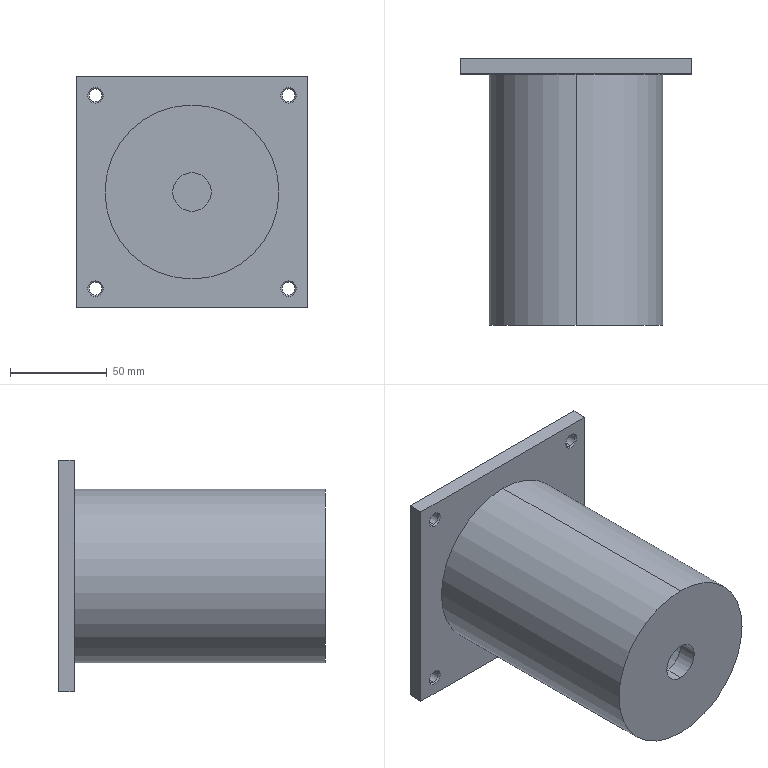Part | SolidWorks | features BaseBody 1 | 1 solid | 39 faces | box 120 x 138 x 120 mm | volume 787135 mm3 | cone 16 | cylinder 14 | plane 9 | commonest cylinder face diameters 6.647 x8 20 x2 40 x2 90 x2
STEP:
#1=CARTESIAN_POINT('',(50.,-0.6765,53.324));
#2=VERTEX_POINT('',#1);
#3=CARTESIAN_POINT('',(50.,-0.6765,46.677));
#4=VERTEX_POINT('',#3);
#5=CARTESIAN_POINT('',(50.,-0.6765,50.));
#6=DIRECTION('',(0.,-1.,0.));
#7=DIRECTION('',(0.,0.,-1.));
#8=AXIS2_PLACEMENT_3D('',#5,#6,#7);
#9=CIRCLE('',#8,3.324);
#10=EDGE_CURVE('',#2,#4,#9,.T.);
#11=ORIENTED_EDGE('',*,*,#10,.T.);
#12=CARTESIAN_POINT('',(50.,0.,46.));
#13=VERTEX_POINT('',#12);
#14=CARTESIAN_POINT('',(50.,0.,46.));
#15=DIRECTION('',(0.,0.7071,-0.7071));
#16=VECTOR('',#15,1000.);
#17=LINE('',#14,#16);
#18=EDGE_CURVE('',#4,#13,#17,.T.);
#19=ORIENTED_EDGE('',*,*,#18,.T.);
#20=CARTESIAN_POINT('',(50.,0.,54.));
#21=VERTEX_POINT('',#20);
#22=CARTESIAN_POINT('',(50.,0.,50.));
#23=DIRECTION('',(0.,-1.,0.));
#24=DIRECTION('',(0.,0.,-1.));
#25=AXIS2_PLACEMENT_3D('',#22,#23,#24);
#26=CIRCLE('',#25,4.);
#27=EDGE_CURVE('',#21,#13,#26,.T.);
#28=ORIENTED_EDGE('',*,*,#27,.F.);
#29=CARTESIAN_POINT('',(50.,0.,54.));
#30=DIRECTION('',(0.,0.7071,0.7071));
#31=VECTOR('',#30,1000.);
#32=LINE('',#29,#31);
#33=EDGE_CURVE('',#2,#21,#32,.T.);
#34=ORIENTED_EDGE('',*,*,#33,.F.);
#35=EDGE_LOOP('',(#11,#19,#28,#34));
#36=FACE_OUTER_BOUND('',#35,.T.);
#37=CARTESIAN_POINT('',(50.,0.,50.));
#38=DIRECTION('',(0.,1.,0.));
#39=DIRECTION('',(0.,0.,1.));
#40=AXIS2_PLACEMENT_3D('',#37,#38,#39);
#41=CONICAL_SURFACE('',#40,4.,0.7854);
#42=ADVANCED_FACE('',(#36),#41,.F.);
#43=CARTESIAN_POINT('',(-50.,-0.6765,53.324));
#44=VERTEX_POINT('',#43);
#45=CARTESIAN_POINT('',(-50.,-0.6765,46.677));
#46=VERTEX_POINT('',#45);
#47=CARTESIAN_POINT('',(-50.,-0.6765,50.));
#48=DIRECTION('',(0.,-1.,0.));
#49=DIRECTION('',(0.,0.,-1.));
#50=AXIS2_PLACEMENT_3D('',#47,#48,#49);
#51=CIRCLE('',#50,3.324);
#52=EDGE_CURVE('',#44,#46,#51,.T.);
#53=ORIENTED_EDGE('',*,*,#52,.T.);
#54=CARTESIAN_POINT('',(-50.,0.,46.));
#55=VERTEX_POINT('',#54);
#56=CARTESIAN_POINT('',(-50.,0.,46.));
#57=DIRECTION('',(0.,0.7071,-0.7071));
#58=VECTOR('',#57,1000.);
#59=LINE('',#56,#58);
#60=EDGE_CURVE('',#46,#55,#59,.T.);
#61=ORIENTED_EDGE('',*,*,#60,.T.);
#62=CARTESIAN_POINT('',(-50.,0.,54.));
#63=VERTEX_POINT('',#62);
#64=CARTESIAN_POINT('',(-50.,0.,50.));
#65=DIRECTION('',(0.,-1.,0.));
#66=DIRECTION('',(0.,0.,-1.));
#67=AXIS2_PLACEMENT_3D('',#64,#65,#66);
#68=CIRCLE('',#67,4.);
#69=EDGE_CURVE('',#63,#55,#68,.T.);
#70=ORIENTED_EDGE('',*,*,#69,.F.);
#71=CARTESIAN_POINT('',(-50.,0.,54.));
#72=DIRECTION('',(0.,0.7071,0.7071));
#73=VECTOR('',#72,1000.);
#74=LINE('',#71,#73);
#75=EDGE_CURVE('',#44,#63,#74,.T.);
#76=ORIENTED_EDGE('',*,*,#75,.F.);
#77=EDGE_LOOP('',(#53,#61,#70,#76));
#78=FACE_OUTER_BOUND('',#77,.T.);
#79=CARTESIAN_POINT('',(-50.,0.,50.));
#80=DIRECTION('',(0.,1.,0.));
#81=DIRECTION('',(0.,0.,1.));
#82=AXIS2_PLACEMENT_3D('',#79,#80,#81);
#83=CONICAL_SURFACE('',#82,4.,0.7854);
#84=ADVANCED_FACE('',(#78),#83,.F.);
#85=CARTESIAN_POINT('',(-50.,-0.6765,-46.677));
#86=VERTEX_POINT('',#85);
#87=CARTESIAN_POINT('',(-50.,-0.6765,-53.324));
#88=VERTEX_POINT('',#87);
#89=CARTESIAN_POINT('',(-50.,-0.6765,-50.));
#90=DIRECTION('',(0.,-1.,0.));
#91=DIRECTION('',(0.,0.,-1.));
#92=AXIS2_PLACEMENT_3D('',#89,#90,#91);
#93=CIRCLE('',#92,3.324);
#94=EDGE_CURVE('',#86,#88,#93,.T.);
#95=ORIENTED_EDGE('',*,*,#94,.T.);
#96=CARTESIAN_POINT('',(-50.,0.,-54.));
#97=VERTEX_POINT('',#96);
#98=CARTESIAN_POINT('',(-50.,0.,-54.));
#99=DIRECTION('',(0.,0.7071,-0.7071));
#100=VECTOR('',#99,1000.);
#101=LINE('',#98,#100);
#102=EDGE_CURVE('',#88,#97,#101,.T.);
#103=ORIENTED_EDGE('',*,*,#102,.T.);
#104=CARTESIAN_POINT('',(-50.,0.,-46.));
#105=VERTEX_POINT('',#104);
#106=CARTESIAN_POINT('',(-50.,0.,-50.));
#107=DIRECTION('',(0.,-1.,0.));
#108=DIRECTION('',(0.,0.,-1.));
#109=AXIS2_PLACEMENT_3D('',#106,#107,#108);
#110=CIRCLE('',#109,4.);
#111=EDGE_CURVE('',#105,#97,#110,.T.);
#112=ORIENTED_EDGE('',*,*,#111,.F.);
#113=CARTESIAN_POINT('',(-50.,0.,-46.));
#114=DIRECTION('',(0.,0.7071,0.7071));
#115=VECTOR('',#114,1000.);
#116=LINE('',#113,#115);
#117=EDGE_CURVE('',#86,#105,#116,.T.);
#118=ORIENTED_EDGE('',*,*,#117,.F.);
#119=EDGE_LOOP('',(#95,#103,#112,#118));
#120=FACE_OUTER_BOUND('',#119,.T.);
#121=CARTESIAN_POINT('',(-50.,0.,-50.));
#122=DIRECTION('',(0.,1.,0.));
#123=DIRECTION('',(0.,0.,1.));
#124=AXIS2_PLACEMENT_3D('',#121,#122,#123);
#125=CONICAL_SURFACE('',#124,4.,0.7854);
#126=ADVANCED_FACE('',(#120),#125,.F.);
#127=CARTESIAN_POINT('',(50.,-0.6765,-46.677));
#128=VERTEX_POINT('',#127);
#129=CARTESIAN_POINT('',(50.,-0.6765,-53.324));
#130=VERTEX_POINT('',#129);
#131=CARTESIAN_POINT('',(50.,-0.6765,-50.));
#132=DIRECTION('',(0.,-1.,0.));
#133=DIRECTION('',(0.,0.,-1.));
#134=AXIS2_PLACEMENT_3D('',#131,#132,#133);
#135=CIRCLE('',#134,3.324);
#136=EDGE_CURVE('',#128,#130,#135,.T.);
#137=ORIENTED_EDGE('',*,*,#136,.T.);
#138=CARTESIAN_POINT('',(50.,0.,-54.));
#139=VERTEX_POINT('',#138);
#140=CARTESIAN_POINT('',(50.,0.,-54.));
#141=DIRECTION('',(0.,0.7071,-0.7071));
#142=VECTOR('',#141,1000.);
#143=LINE('',#140,#142);
#144=EDGE_CURVE('',#130,#139,#143,.T.);
#145=ORIENTED_EDGE('',*,*,#144,.T.);
#146=CARTESIAN_POINT('',(50.,0.,-46.));
#147=VERTEX_POINT('',#146);
#148=CARTESIAN_POINT('',(50.,0.,-50.));
#149=DIRECTION('',(0.,-1.,0.));
#150=DIRECTION('',(0.,0.,-1.));
#151=AXIS2_PLACEMENT_3D('',#148,#149,#150);
#152=CIRCLE('',#151,4.);
#153=EDGE_CURVE('',#147,#139,#152,.T.);
#154=ORIENTED_EDGE('',*,*,#153,.F.);
#155=CARTESIAN_POINT('',(50.,0.,-46.));
#156=DIRECTION('',(0.,0.7071,0.7071));
#157=VECTOR('',#156,1000.);
#158=LINE('',#155,#157);
#159=EDGE_CURVE('',#128,#147,#158,.T.);
#160=ORIENTED_EDGE('',*,*,#159,.F.);
#161=EDGE_LOOP('',(#137,#145,#154,#160));
#162=FACE_OUTER_BOUND('',#161,.T.);
#163=CARTESIAN_POINT('',(50.,0.,-50.));
#164=DIRECTION('',(0.,1.,0.));
#165=DIRECTION('',(0.,0.,1.));
#166=AXIS2_PLACEMENT_3D('',#163,#164,#165);
#167=CONICAL_SURFACE('',#166,4.,0.7854);
#168=ADVANCED_FACE('',(#162),#167,.F.);
#169=ORIENTED_EDGE('',*,*,#10,.F.);
#170=CARTESIAN_POINT('',(50.,-7.324,53.324));
#171=VERTEX_POINT('',#170);
#172=CARTESIAN_POINT('',(50.,-8.,53.324));
#173=DIRECTION('',(0.,-1.,0.));
#174=VECTOR('',#173,1000.);
#175=LINE('',#172,#174);
#176=EDGE_CURVE('',#2,#171,#175,.T.);
#177=ORIENTED_EDGE('',*,*,#176,.T.);
#178=CARTESIAN_POINT('',(50.,-7.324,46.677));
#179=VERTEX_POINT('',#178);
#180=CARTESIAN_POINT('',(50.,-7.324,50.));
#181=DIRECTION('',(0.,-1.,0.));
#182=DIRECTION('',(0.,0.,-1.));
#183=AXIS2_PLACEMENT_3D('',#180,#181,#182);
#184=CIRCLE('',#183,3.324);
#185=EDGE_CURVE('',#171,#179,#184,.T.);
#186=ORIENTED_EDGE('',*,*,#185,.T.);
#187=CARTESIAN_POINT('',(50.,-8.,46.677));
#188=DIRECTION('',(0.,-1.,0.));
#189=VECTOR('',#188,1000.);
#190=LINE('',#187,#189);
#191=EDGE_CURVE('',#4,#179,#190,.T.);
#192=ORIENTED_EDGE('',*,*,#191,.F.);
#193=EDGE_LOOP('',(#169,#177,#186,#192));
#194=FACE_OUTER_BOUND('',#193,.T.);
#195=CARTESIAN_POINT('',(50.,-8.,50.));
#196=DIRECTION('',(0.,-1.,0.));
#197=DIRECTION('',(0.,0.,-1.));
#198=AXIS2_PLACEMENT_3D('',#195,#196,#197);
#199=CYLINDRICAL_SURFACE('',#198,3.324);
#200=ADVANCED_FACE('',(#194),#199,.F.);
#201=ORIENTED_EDGE('',*,*,#52,.F.);
#202=CARTESIAN_POINT('',(-50.,-7.324,53.324));
#203=VERTEX_POINT('',#202);
#204=CARTESIAN_POINT('',(-50.,-8.,53.324));
#205=DIRECTION('',(0.,-1.,0.));
#206=VECTOR('',#205,1000.);
#207=LINE('',#204,#206);
#208=EDGE_CURVE('',#44,#203,#207,.T.);
#209=ORIENTED_EDGE('',*,*,#208,.T.);
#210=CARTESIAN_POINT('',(-50.,-7.324,46.677));
#211=VERTEX_POINT('',#210);
#212=CARTESIAN_POINT('',(-50.,-7.324,50.));
#213=DIRECTION('',(0.,-1.,0.));
#214=DIRECTION('',(0.,0.,-1.));
#215=AXIS2_PLACEMENT_3D('',#212,#213,#214);
#216=CIRCLE('',#215,3.324);
#217=EDGE_CURVE('',#203,#211,#216,.T.);
#218=ORIENTED_EDGE('',*,*,#217,.T.);
#219=CARTESIAN_POINT('',(-50.,-8.,46.677));
#220=DIRECTION('',(0.,-1.,0.));
#221=VECTOR('',#220,1000.);
#222=LINE('',#219,#221);
#223=EDGE_CURVE('',#46,#211,#222,.T.);
#224=ORIENTED_EDGE('',*,*,#223,.F.);
#225=EDGE_LOOP('',(#201,#209,#218,#224));
#226=FACE_OUTER_BOUND('',#225,.T.);
#227=CARTESIAN_POINT('',(-50.,-8.,50.));
#228=DIRECTION('',(0.,-1.,0.));
#229=DIRECTION('',(0.,0.,-1.));
#230=AXIS2_PLACEMENT_3D('',#227,#228,#229);
#231=CYLINDRICAL_SURFACE('',#230,3.324);
#232=ADVANCED_FACE('',(#226),#231,.F.);
#233=ORIENTED_EDGE('',*,*,#94,.F.);
#234=CARTESIAN_POINT('',(-50.,-7.324,-46.677));
#235=VERTEX_POINT('',#234);
#236=CARTESIAN_POINT('',(-50.,-8.,-46.677));
#237=DIRECTION('',(0.,-1.,0.));
#238=VECTOR('',#237,1000.);
#239=LINE('',#236,#238);
#240=EDGE_CURVE('',#86,#235,#239,.T.);
#241=ORIENTED_EDGE('',*,*,#240,.T.);
#242=CARTESIAN_POINT('',(-50.,-7.324,-53.324));
#243=VERTEX_POINT('',#242);
#244=CARTESIAN_POINT('',(-50.,-7.324,-50.));
#245=DIRECTION('',(0.,-1.,0.));
#246=DIRECTION('',(0.,0.,-1.));
#247=AXIS2_PLACEMENT_3D('',#244,#245,#246);
#248=CIRCLE('',#247,3.324);
#249=EDGE_CURVE('',#235,#243,#248,.T.);
#250=ORIENTED_EDGE('',*,*,#249,.T.);
#251=CARTESIAN_POINT('',(-50.,-8.,-53.324));
#252=DIRECTION('',(0.,-1.,0.));
#253=VECTOR('',#252,1000.);
#254=LINE('',#251,#253);
#255=EDGE_CURVE('',#88,#243,#254,.T.);
#256=ORIENTED_EDGE('',*,*,#255,.F.);
#257=EDGE_LOOP('',(#233,#241,#250,#256));
#258=FACE_OUTER_BOUND('',#257,.T.);
#259=CARTESIAN_POINT('',(-50.,-8.,-50.));
#260=DIRECTION('',(0.,-1.,0.));
#261=DIRECTION('',(0.,0.,-1.));
#262=AXIS2_PLACEMENT_3D('',#259,#260,#261);
#263=CYLINDRICAL_SURFACE('',#262,3.324);
#264=ADVANCED_FACE('',(#258),#263,.F.);
#265=ORIENTED_EDGE('',*,*,#136,.F.);
#266=CARTESIAN_POINT('',(50.,-7.324,-46.677));
#267=VERTEX_POINT('',#266);
#268=CARTESIAN_POINT('',(50.,-8.,-46.677));
#269=DIRECTION('',(0.,-1.,0.));
#270=VECTOR('',#269,1000.);
#271=LINE('',#268,#270);
#272=EDGE_CURVE('',#128,#267,#271,.T.);
#273=ORIENTED_EDGE('',*,*,#272,.T.);
#274=CARTESIAN_POINT('',(50.,-7.324,-53.324));
#275=VERTEX_POINT('',#274);
#276=CARTESIAN_POINT('',(50.,-7.324,-50.));
#277=DIRECTION('',(0.,-1.,0.));
#278=DIRECTION('',(0.,0.,-1.));
#279=AXIS2_PLACEMENT_3D('',#276,#277,#278);
#280=CIRCLE('',#279,3.324);
#281=EDGE_CURVE('',#267,#275,#280,.T.);
#282=ORIENTED_EDGE('',*,*,#281,.T.);
#283=CARTESIAN_POINT('',(50.,-8.,-53.324));
#284=DIRECTION('',(0.,-1.,0.));
#285=VECTOR('',#284,1000.);
#286=LINE('',#283,#285);
#287=EDGE_CURVE('',#130,#275,#286,.T.);
#288=ORIENTED_EDGE('',*,*,#287,.F.);
#289=EDGE_LOOP('',(#265,#273,#282,#288));
#290=FACE_OUTER_BOUND('',#289,.T.);
#291=CARTESIAN_POINT('',(50.,-8.,-50.));
#292=DIRECTION('',(0.,-1.,0.));
#293=DIRECTION('',(0.,0.,-1.));
#294=AXIS2_PLACEMENT_3D('',#291,#292,#293);
#295=CYLINDRICAL_SURFACE('',#294,3.324);
#296=ADVANCED_FACE('',(#290),#295,.F.);
#297=ORIENTED_EDGE('',*,*,#185,.F.);
#298=CARTESIAN_POINT('',(50.,-8.,54.));
#299=VERTEX_POINT('',#298);
#300=CARTESIAN_POINT('',(50.,-7.324,53.324));
#301=DIRECTION('',(0.,-0.7071,0.7071));
#302=VECTOR('',#301,1000.);
#303=LINE('',#300,#302);
#304=EDGE_CURVE('',#171,#299,#303,.T.);
#305=ORIENTED_EDGE('',*,*,#304,.T.);
#306=CARTESIAN_POINT('',(50.,-8.,46.));
#307=VERTEX_POINT('',#306);
#308=CARTESIAN_POINT('',(50.,-8.,50.));
#309=DIRECTION('',(0.,-1.,0.));
#310=DIRECTION('',(0.,0.,-1.));
#311=AXIS2_PLACEMENT_3D('',#308,#309,#310);
#312=CIRCLE('',#311,4.);
#313=EDGE_CURVE('',#299,#307,#312,.T.);
#314=ORIENTED_EDGE('',*,*,#313,.T.);
#315=CARTESIAN_POINT('',(50.,-7.324,46.677));
#316=DIRECTION('',(0.,-0.7071,-0.7071));
#317=VECTOR('',#316,1000.);
#318=LINE('',#315,#317);
#319=EDGE_CURVE('',#179,#307,#318,.T.);
#320=ORIENTED_EDGE('',*,*,#319,.F.);
#321=EDGE_LOOP('',(#297,#305,#314,#320));
#322=FACE_OUTER_BOUND('',#321,.T.);
#323=CARTESIAN_POINT('',(50.,-7.324,50.));
#324=DIRECTION('',(0.,-1.,0.));
#325=DIRECTION('',(0.,0.,-1.));
#326=AXIS2_PLACEMENT_3D('',#323,#324,#325);
#327=CONICAL_SURFACE('',#326,3.324,0.7854);
#328=ADVANCED_FACE('',(#322),#327,.F.);
#329=ORIENTED_EDGE('',*,*,#217,.F.);
#330=CARTESIAN_POINT('',(-50.,-8.,54.));
#331=VERTEX_POINT('',#330);
#332=CARTESIAN_POINT('',(-50.,-7.324,53.324));
#333=DIRECTION('',(0.,-0.7071,0.7071));
#334=VECTOR('',#333,1000.);
#335=LINE('',#332,#334);
#336=EDGE_CURVE('',#203,#331,#335,.T.);
#337=ORIENTED_EDGE('',*,*,#336,.T.);
#338=CARTESIAN_POINT('',(-50.,-8.,46.));
#339=VERTEX_POINT('',#338);
#340=CARTESIAN_POINT('',(-50.,-8.,50.));
#341=DIRECTION('',(0.,-1.,0.));
#342=DIRECTION('',(0.,0.,-1.));
#343=AXIS2_PLACEMENT_3D('',#340,#341,#342);
#344=CIRCLE('',#343,4.);
#345=EDGE_CURVE('',#331,#339,#344,.T.);
#346=ORIENTED_EDGE('',*,*,#345,.T.);
#347=CARTESIAN_POINT('',(-50.,-7.324,46.677));
#348=DIRECTION('',(0.,-0.7071,-0.7071));
#349=VECTOR('',#348,1000.);
#350=LINE('',#347,#349);
#351=EDGE_CURVE('',#211,#339,#350,.T.);
#352=ORIENTED_EDGE('',*,*,#351,.F.);
#353=EDGE_LOOP('',(#329,#337,#346,#352));
#354=FACE_OUTER_BOUND('',#353,.T.);
#355=CARTESIAN_POINT('',(-50.,-7.324,50.));
#356=DIRECTION('',(0.,-1.,0.));
#357=DIRECTION('',(0.,0.,-1.));
#358=AXIS2_PLACEMENT_3D('',#355,#356,#357);
#359=CONICAL_SURFACE('',#358,3.324,0.7854);
#360=ADVANCED_FACE('',(#354),#359,.F.);
#361=ORIENTED_EDGE('',*,*,#249,.F.);
#362=CARTESIAN_POINT('',(-50.,-8.,-46.));
#363=VERTEX_POINT('',#362);
#364=CARTESIAN_POINT('',(-50.,-7.324,-46.677));
#365=DIRECTION('',(0.,-0.7071,0.7071));
#366=VECTOR('',#365,1000.);
#367=LINE('',#364,#366);
#368=EDGE_CURVE('',#235,#363,#367,.T.);
#369=ORIENTED_EDGE('',*,*,#368,.T.);
#370=CARTESIAN_POINT('',(-50.,-8.,-54.));
#371=VERTEX_POINT('',#370);
#372=CARTESIAN_POINT('',(-50.,-8.,-50.));
#373=DIRECTION('',(0.,-1.,0.));
#374=DIRECTION('',(0.,0.,-1.));
#375=AXIS2_PLACEMENT_3D('',#372,#373,#374);
#376=CIRCLE('',#375,4.);
#377=EDGE_CURVE('',#363,#371,#376,.T.);
#378=ORIENTED_EDGE('',*,*,#377,.T.);
#379=CARTESIAN_POINT('',(-50.,-7.324,-53.324));
#380=DIRECTION('',(0.,-0.7071,-0.7071));
#381=VECTOR('',#380,1000.);
#382=LINE('',#379,#381);
#383=EDGE_CURVE('',#243,#371,#382,.T.);
#384=ORIENTED_EDGE('',*,*,#383,.F.);
#385=EDGE_LOOP('',(#361,#369,#378,#384));
#386=FACE_OUTER_BOUND('',#385,.T.);
#387=CARTESIAN_POINT('',(-50.,-7.324,-50.));
#388=DIRECTION('',(0.,-1.,0.));
#389=DIRECTION('',(0.,0.,-1.));
#390=AXIS2_PLACEMENT_3D('',#387,#388,#389);
#391=CONICAL_SURFACE('',#390,3.324,0.7854);
#392=ADVANCED_FACE('',(#386),#391,.F.);
#393=ORIENTED_EDGE('',*,*,#281,.F.);
#394=CARTESIAN_POINT('',(50.,-8.,-46.));
#395=VERTEX_POINT('',#394);
#396=CARTESIAN_POINT('',(50.,-7.324,-46.677));
#397=DIRECTION('',(0.,-0.7071,0.7071));
#398=VECTOR('',#397,1000.);
#399=LINE('',#396,#398);
#400=EDGE_CURVE('',#267,#395,#399,.T.);
#401=ORIENTED_EDGE('',*,*,#400,.T.);
#402=CARTESIAN_POINT('',(50.,-8.,-54.));
#403=VERTEX_POINT('',#402);
#404=CARTESIAN_POINT('',(50.,-8.,-50.));
#405=DIRECTION('',(0.,-1.,0.));
#406=DIRECTION('',(0.,0.,-1.));
#407=AXIS2_PLACEMENT_3D('',#404,#405,#406);
#408=CIRCLE('',#407,4.);
#409=EDGE_CURVE('',#395,#403,#408,.T.);
#410=ORIENTED_EDGE('',*,*,#409,.T.);
#411=CARTESIAN_POINT('',(50.,-7.324,-53.324));
#412=DIRECTION('',(0.,-0.7071,-0.7071));
#413=VECTOR('',#412,1000.);
#414=LINE('',#411,#413);
#415=EDGE_CURVE('',#275,#403,#414,.T.);
#416=ORIENTED_EDGE('',*,*,#415,.F.);
#417=EDGE_LOOP('',(#393,#401,#410,#416));
#418=FACE_OUTER_BOUND('',#417,.T.);
#419=CARTESIAN_POINT('',(50.,-7.324,-50.));
#420=DIRECTION('',(0.,-1.,0.));
#421=DIRECTION('',(0.,0.,-1.));
#422=AXIS2_PLACEMENT_3D('',#419,#420,#421);
#423=CONICAL_SURFACE('',#422,3.324,0.7854);
#424=ADVANCED_FACE('',(#418),#423,.F.);
#425=CARTESIAN_POINT('',(0.,-128.,-20.));
#426=VERTEX_POINT('',#425);
#427=CARTESIAN_POINT('',(0.,-128.,20.));
#428=VERTEX_POINT('',#427);
#429=CARTESIAN_POINT('',(0.,-128.,0.));
#430=DIRECTION('',(0.,1.,0.));
#431=DIRECTION('',(1.,0.,0.));
#432=AXIS2_PLACEMENT_3D('',#429,#430,#431);
#433=CIRCLE('',#432,20.);
#434=EDGE_CURVE('',#426,#428,#433,.T.);
#435=ORIENTED_EDGE('',*,*,#434,.F.);
#436=CARTESIAN_POINT('',(0.,-8.,-20.));
#437=VERTEX_POINT('',#436);
#438=CARTESIAN_POINT('',(0.,-128.,-20.));
#439=DIRECTION('',(0.,1.,0.));
#440=VECTOR('',#439,1000.);
#441=LINE('',#438,#440);
#442=EDGE_CURVE('',#426,#437,#441,.T.);
#443=ORIENTED_EDGE('',*,*,#442,.T.);
#444=CARTESIAN_POINT('',(0.,-8.,20.));
#445=VERTEX_POINT('',#444);
#446=CARTESIAN_POINT('',(0.,-8.,0.));
#447=DIRECTION('',(0.,1.,0.));
#448=DIRECTION('',(1.,0.,0.));
#449=AXIS2_PLACEMENT_3D('',#446,#447,#448);
#450=CIRCLE('',#449,20.);
#451=EDGE_CURVE('',#437,#445,#450,.T.);
#452=ORIENTED_EDGE('',*,*,#451,.T.);
#453=CARTESIAN_POINT('',(0.,-128.,20.));
#454=DIRECTION('',(0.,1.,0.));
#455=VECTOR('',#454,1000.);
#456=LINE('',#453,#455);
#457=EDGE_CURVE('',#428,#445,#456,.T.);
#458=ORIENTED_EDGE('',*,*,#457,.F.);
#459=EDGE_LOOP('',(#435,#443,#452,#458));
#460=FACE_OUTER_BOUND('',#459,.T.);
#461=CARTESIAN_POINT('',(0.,-128.,0.));
#462=DIRECTION('',(0.,1.,0.));
#463=DIRECTION('',(0.,0.,1.));
#464=AXIS2_PLACEMENT_3D('',#461,#462,#463);
#465=CYLINDRICAL_SURFACE('',#464,20.);
#466=ADVANCED_FACE('',(#460),#465,.F.);
#467=CARTESIAN_POINT('',(0.,-138.,45.));
#468=VERTEX_POINT('',#467);
#469=CARTESIAN_POINT('',(0.,-138.,-45.));
#470=VERTEX_POINT('',#469);
#471=CARTESIAN_POINT('',(0.,-138.,0.));
#472=DIRECTION('',(0.,1.,0.));
#473=DIRECTION('',(1.,0.,0.));
#474=AXIS2_PLACEMENT_3D('',#471,#472,#473);
#475=CIRCLE('',#474,45.);
#476=EDGE_CURVE('',#468,#470,#475,.T.);
#477=ORIENTED_EDGE('',*,*,#476,.T.);
#478=CARTESIAN_POINT('',(0.,-8.,-45.));
#479=VERTEX_POINT('',#478);
#480=CARTESIAN_POINT('',(0.,-138.,-45.));
#481=DIRECTION('',(0.,1.,0.));
#482=VECTOR('',#481,1000.);
#483=LINE('',#480,#482);
#484=EDGE_CURVE('',#470,#479,#483,.T.);
#485=ORIENTED_EDGE('',*,*,#484,.T.);
#486=CARTESIAN_POINT('',(0.,-8.,45.));
#487=VERTEX_POINT('',#486);
#488=CARTESIAN_POINT('',(0.,-8.,0.));
#489=DIRECTION('',(0.,1.,0.));
#490=DIRECTION('',(1.,0.,0.));
#491=AXIS2_PLACEMENT_3D('',#488,#489,#490);
#492=CIRCLE('',#491,45.);
#493=EDGE_CURVE('',#487,#479,#492,.T.);
#494=ORIENTED_EDGE('',*,*,#493,.F.);
#495=CARTESIAN_POINT('',(0.,-138.,45.));
#496=DIRECTION('',(0.,1.,0.));
#497=VECTOR('',#496,1000.);
#498=LINE('',#495,#497);
#499=EDGE_CURVE('',#468,#487,#498,.T.);
#500=ORIENTED_EDGE('',*,*,#499,.F.);
#501=EDGE_LOOP('',(#477,#485,#494,#500));
#502=FACE_OUTER_BOUND('',#501,.T.);
#503=CARTESIAN_POINT('',(0.,-138.,0.));
#504=DIRECTION('',(0.,1.,0.));
#505=DIRECTION('',(0.,0.,1.));
#506=AXIS2_PLACEMENT_3D('',#503,#504,#505);
#507=CYLINDRICAL_SURFACE('',#506,45.);
#508=ADVANCED_FACE('',(#502),#507,.T.);
#509=CARTESIAN_POINT('',(0.,-138.,-10.));
#510=VERTEX_POINT('',#509);
#511=CARTESIAN_POINT('',(0.,-138.,10.));
#512=VERTEX_POINT('',#511);
#513=CARTESIAN_POINT('',(0.,-138.,0.));
#514=DIRECTION('',(0.,1.,0.));
#515=DIRECTION('',(0.,0.,1.));
#516=AXIS2_PLACEMENT_3D('',#513,#514,#515);
#517=CIRCLE('',#516,10.);
#518=EDGE_CURVE('',#510,#512,#517,.T.);
#519=ORIENTED_EDGE('',*,*,#518,.F.);
#520=CARTESIAN_POINT('',(0.,-128.,-10.));
#521=VERTEX_POINT('',#520);
#522=CARTESIAN_POINT('',(0.,-138.5,-10.));
#523=DIRECTION('',(0.,1.,0.));
#524=VECTOR('',#523,1000.);
#525=LINE('',#522,#524);
#526=EDGE_CURVE('',#510,#521,#525,.T.);
#527=ORIENTED_EDGE('',*,*,#526,.T.);
#528=CARTESIAN_POINT('',(0.,-128.,10.));
#529=VERTEX_POINT('',#528);
#530=CARTESIAN_POINT('',(0.,-128.,0.));
#531=DIRECTION('',(0.,-1.,0.));
#532=DIRECTION('',(0.,0.,1.));
#533=AXIS2_PLACEMENT_3D('',#530,#531,#532);
#534=CIRCLE('',#533,10.);
#535=EDGE_CURVE('',#529,#521,#534,.T.);
#536=ORIENTED_EDGE('',*,*,#535,.F.);
#537=CARTESIAN_POINT('',(0.,-138.5,10.));
#538=DIRECTION('',(0.,1.,0.));
#539=VECTOR('',#538,1000.);
#540=LINE('',#537,#539);
#541=EDGE_CURVE('',#512,#529,#540,.T.);
#542=ORIENTED_EDGE('',*,*,#541,.F.);
#543=EDGE_LOOP('',(#519,#527,#536,#542));
#544=FACE_OUTER_BOUND('',#543,.T.);
#545=CARTESIAN_POINT('',(0.,-138.5,0.));
#546=DIRECTION('',(0.,1.,0.));
#547=DIRECTION('',(0.,0.,1.));
#548=AXIS2_PLACEMENT_3D('',#545,#546,#547);
#549=CYLINDRICAL_SURFACE('',#548,10.);
#550=ADVANCED_FACE('',(#544),#549,.F.);
#551=ORIENTED_EDGE('',*,*,#526,.F.);
#552=CARTESIAN_POINT('',(0.,-138.,0.));
#553=DIRECTION('',(0.,1.,0.));
#554=DIRECTION('',(0.,0.,1.));
#555=AXIS2_PLACEMENT_3D('',#552,#553,#554);
#556=CIRCLE('',#555,10.);
#557=EDGE_CURVE('',#512,#510,#556,.T.);
#558=ORIENTED_EDGE('',*,*,#557,.F.);
#559=ORIENTED_EDGE('',*,*,#541,.T.);
#560=CARTESIAN_POINT('',(0.,-128.,0.));
#561=DIRECTION('',(0.,-1.,0.));
#562=DIRECTION('',(0.,0.,1.));
#563=AXIS2_PLACEMENT_3D('',#560,#561,#562);
#564=CIRCLE('',#563,10.);
#565=EDGE_CURVE('',#521,#529,#564,.T.);
#566=ORIENTED_EDGE('',*,*,#565,.F.);
#567=EDGE_LOOP('',(#551,#558,#559,#566));
#568=FACE_OUTER_BOUND('',#567,.T.);
#569=CARTESIAN_POINT('',(0.,-138.5,0.));
#570=DIRECTION('',(0.,1.,0.));
#571=DIRECTION('',(0.,0.,1.));
#572=AXIS2_PLACEMENT_3D('',#569,#570,#571);
#573=CYLINDRICAL_SURFACE('',#572,10.);
#574=ADVANCED_FACE('',(#568),#573,.F.);
#575=ORIENTED_EDGE('',*,*,#557,.T.);
#576=ORIENTED_EDGE('',*,*,#518,.T.);
#577=EDGE_LOOP('',(#575,#576));
#578=FACE_BOUND('',#577,.T.);
#579=ORIENTED_EDGE('',*,*,#476,.F.);
#580=CARTESIAN_POINT('',(0.,-138.,0.));
#581=DIRECTION('',(0.,1.,0.));
#582=DIRECTION('',(1.,0.,0.));
#583=AXIS2_PLACEMENT_3D('',#580,#581,#582);
#584=CIRCLE('',#583,45.);
#585=EDGE_CURVE('',#470,#468,#584,.T.);
#586=ORIENTED_EDGE('',*,*,#585,.F.);
#587=EDGE_LOOP('',(#579,#586));
#588=FACE_OUTER_BOUND('',#587,.T.);
#589=CARTESIAN_POINT('',(0.,-138.,0.));
#590=DIRECTION('',(0.,1.,0.));
#591=DIRECTION('',(0.,0.,1.));
#592=AXIS2_PLACEMENT_3D('',#589,#590,#591);
#593=PLANE('',#592);
#594=ADVANCED_FACE('',(#578,#588),#593,.F.);
#595=CARTESIAN_POINT('',(0.,-128.,0.));
#596=DIRECTION('',(0.,1.,0.));
#597=DIRECTION('',(1.,0.,0.));
#598=AXIS2_PLACEMENT_3D('',#595,#596,#597);
#599=CIRCLE('',#598,20.);
#600=EDGE_CURVE('',#428,#426,#599,.T.);
#601=ORIENTED_EDGE('',*,*,#600,.T.);
#602=ORIENTED_EDGE('',*,*,#434,.T.);
#603=EDGE_LOOP('',(#601,#602));
#604=FACE_OUTER_BOUND('',#603,.T.);
#605=ORIENTED_EDGE('',*,*,#535,.T.);
#606=ORIENTED_EDGE('',*,*,#565,.T.);
#607=EDGE_LOOP('',(#605,#606));
#608=FACE_BOUND('',#607,.T.);
#609=CARTESIAN_POINT('',(0.,-128.,0.));
#610=DIRECTION('',(0.,1.,0.));
#611=DIRECTION('',(0.,0.,1.));
#612=AXIS2_PLACEMENT_3D('',#609,#610,#611);
#613=PLANE('',#612);
#614=ADVANCED_FACE('',(#604,#608),#613,.T.);
#615=ORIENTED_EDGE('',*,*,#484,.F.);
#616=ORIENTED_EDGE('',*,*,#585,.T.);
#617=ORIENTED_EDGE('',*,*,#499,.T.);
#618=CARTESIAN_POINT('',(0.,-8.,0.));
#619=DIRECTION('',(0.,1.,0.));
#620=DIRECTION('',(1.,0.,0.));
#621=AXIS2_PLACEMENT_3D('',#618,#619,#620);
#622=CIRCLE('',#621,45.);
#623=EDGE_CURVE('',#479,#487,#622,.T.);
#624=ORIENTED_EDGE('',*,*,#623,.F.);
#625=EDGE_LOOP('',(#615,#616,#617,#624));
#626=FACE_OUTER_BOUND('',#625,.T.);
#627=CARTESIAN_POINT('',(0.,-138.,0.));
#628=DIRECTION('',(0.,1.,0.));
#629=DIRECTION('',(0.,0.,1.));
#630=AXIS2_PLACEMENT_3D('',#627,#628,#629);
#631=CYLINDRICAL_SURFACE('',#630,45.);
#632=ADVANCED_FACE('',(#626),#631,.T.);
#633=ORIENTED_EDGE('',*,*,#442,.F.);
#634=ORIENTED_EDGE('',*,*,#600,.F.);
#635=ORIENTED_EDGE('',*,*,#457,.T.);
#636=CARTESIAN_POINT('',(0.,-8.,0.));
#637=DIRECTION('',(0.,1.,0.));
#638=DIRECTION('',(1.,0.,0.));
#639=AXIS2_PLACEMENT_3D('',#636,#637,#638);
#640=CIRCLE('',#639,20.);
#641=EDGE_CURVE('',#445,#437,#640,.T.);
#642=ORIENTED_EDGE('',*,*,#641,.T.);
#643=EDGE_LOOP('',(#633,#634,#635,#642));
#644=FACE_OUTER_BOUND('',#643,.T.);
#645=CARTESIAN_POINT('',(0.,-128.,0.));
#646=DIRECTION('',(0.,1.,0.));
#647=DIRECTION('',(0.,0.,1.));
#648=AXIS2_PLACEMENT_3D('',#645,#646,#647);
#649=CYLINDRICAL_SURFACE('',#648,20.);
#650=ADVANCED_FACE('',(#644),#649,.F.);
#651=CARTESIAN_POINT('',(50.,-8.,-50.));
#652=DIRECTION('',(0.,-1.,0.));
#653=DIRECTION('',(0.,0.,-1.));
#654=AXIS2_PLACEMENT_3D('',#651,#652,#653);
#655=CIRCLE('',#654,4.);
#656=EDGE_CURVE('',#403,#395,#655,.T.);
#657=ORIENTED_EDGE('',*,*,#656,.F.);
#658=ORIENTED_EDGE('',*,*,#409,.F.);
#659=EDGE_LOOP('',(#657,#658));
#660=FACE_BOUND('',#659,.T.);
#661=CARTESIAN_POINT('',(-50.,-8.,-50.));
#662=DIRECTION('',(0.,-1.,0.));
#663=DIRECTION('',(0.,0.,-1.));
#664=AXIS2_PLACEMENT_3D('',#661,#662,#663);
#665=CIRCLE('',#664,4.);
#666=EDGE_CURVE('',#371,#363,#665,.T.);
#667=ORIENTED_EDGE('',*,*,#666,.F.);
#668=ORIENTED_EDGE('',*,*,#377,.F.);
#669=EDGE_LOOP('',(#667,#668));
#670=FACE_BOUND('',#669,.T.);
#671=CARTESIAN_POINT('',(-50.,-8.,50.));
#672=DIRECTION('',(0.,-1.,0.));
#673=DIRECTION('',(0.,0.,-1.));
#674=AXIS2_PLACEMENT_3D('',#671,#672,#673);
#675=CIRCLE('',#674,4.);
#676=EDGE_CURVE('',#339,#331,#675,.T.);
#677=ORIENTED_EDGE('',*,*,#676,.F.);
#678=ORIENTED_EDGE('',*,*,#345,.F.);
#679=EDGE_LOOP('',(#677,#678));
#680=FACE_BOUND('',#679,.T.);
#681=CARTESIAN_POINT('',(50.,-8.,50.));
#682=DIRECTION('',(0.,-1.,0.));
#683=DIRECTION('',(0.,0.,-1.));
#684=AXIS2_PLACEMENT_3D('',#681,#682,#683);
#685=CIRCLE('',#684,4.);
#686=EDGE_CURVE('',#307,#299,#685,.T.);
#687=ORIENTED_EDGE('',*,*,#686,.F.);
#688=ORIENTED_EDGE('',*,*,#313,.F.);
#689=EDGE_LOOP('',(#687,#688));
#690=FACE_BOUND('',#689,.T.);
#691=ORIENTED_EDGE('',*,*,#493,.T.);
#692=ORIENTED_EDGE('',*,*,#623,.T.);
#693=EDGE_LOOP('',(#691,#692));
#694=FACE_BOUND('',#693,.T.);
#695=CARTESIAN_POINT('',(60.,-8.,-60.));
#696=VERTEX_POINT('',#695);
#697=CARTESIAN_POINT('',(-60.,-8.,-60.));
#698=VERTEX_POINT('',#697);
#699=CARTESIAN_POINT('',(60.,-8.,-60.));
#700=DIRECTION('',(-1.,0.,0.));
#701=VECTOR('',#700,1000.);
#702=LINE('',#699,#701);
#703=EDGE_CURVE('',#696,#698,#702,.T.);
#704=ORIENTED_EDGE('',*,*,#703,.F.);
#705=CARTESIAN_POINT('',(60.,-8.,60.));
#706=VERTEX_POINT('',#705);
#707=CARTESIAN_POINT('',(60.,-8.,60.));
#708=DIRECTION('',(0.,0.,-1.));
#709=VECTOR('',#708,1000.);
#710=LINE('',#707,#709);
#711=EDGE_CURVE('',#706,#696,#710,.T.);
#712=ORIENTED_EDGE('',*,*,#711,.F.);
#713=CARTESIAN_POINT('',(-60.,-8.,60.));
#714=VERTEX_POINT('',#713);
#715=CARTESIAN_POINT('',(-60.,-8.,60.));
#716=DIRECTION('',(1.,0.,0.));
#717=VECTOR('',#716,1000.);
#718=LINE('',#715,#717);
#719=EDGE_CURVE('',#714,#706,#718,.T.);
#720=ORIENTED_EDGE('',*,*,#719,.F.);
#721=CARTESIAN_POINT('',(-60.,-8.,-60.));
#722=DIRECTION('',(0.,0.,1.));
#723=VECTOR('',#722,1000.);
#724=LINE('',#721,#723);
#725=EDGE_CURVE('',#698,#714,#724,.T.);
#726=ORIENTED_EDGE('',*,*,#725,.F.);
#727=EDGE_LOOP('',(#704,#712,#720,#726));
#728=FACE_OUTER_BOUND('',#727,.T.);
#729=CARTESIAN_POINT('',(0.,-8.,0.));
#730=DIRECTION('',(0.,1.,0.));
#731=DIRECTION('',(0.,0.,1.));
#732=AXIS2_PLACEMENT_3D('',#729,#730,#731);
#733=PLANE('',#732);
#734=ADVANCED_FACE('',(#660,#670,#680,#690,#694,#728),#733,.F.);
#735=ORIENTED_EDGE('',*,*,#641,.F.);
#736=ORIENTED_EDGE('',*,*,#451,.F.);
#737=EDGE_LOOP('',(#735,#736));
#738=FACE_OUTER_BOUND('',#737,.T.);
#739=CARTESIAN_POINT('',(0.,-8.,0.));
#740=DIRECTION('',(0.,1.,0.));
#741=DIRECTION('',(0.,0.,1.));
#742=AXIS2_PLACEMENT_3D('',#739,#740,#741);
#743=PLANE('',#742);
#744=ADVANCED_FACE('',(#738),#743,.F.);
#745=ORIENTED_EDGE('',*,*,#400,.F.);
#746=CARTESIAN_POINT('',(50.,-7.324,-50.));
#747=DIRECTION('',(0.,-1.,0.));
#748=DIRECTION('',(0.,0.,-1.));
#749=AXIS2_PLACEMENT_3D('',#746,#747,#748);
#750=CIRCLE('',#749,3.324);
#751=EDGE_CURVE('',#275,#267,#750,.T.);
#752=ORIENTED_EDGE('',*,*,#751,.F.);
#753=ORIENTED_EDGE('',*,*,#415,.T.);
#754=ORIENTED_EDGE('',*,*,#656,.T.);
#755=EDGE_LOOP('',(#745,#752,#753,#754));
#756=FACE_OUTER_BOUND('',#755,.T.);
#757=CARTESIAN_POINT('',(50.,-7.324,-50.));
#758=DIRECTION('',(0.,-1.,0.));
#759=DIRECTION('',(0.,0.,-1.));
#760=AXIS2_PLACEMENT_3D('',#757,#758,#759);
#761=CONICAL_SURFACE('',#760,3.324,0.7854);
#762=ADVANCED_FACE('',(#756),#761,.F.);
#763=ORIENTED_EDGE('',*,*,#368,.F.);
#764=CARTESIAN_POINT('',(-50.,-7.324,-50.));
#765=DIRECTION('',(0.,-1.,0.));
#766=DIRECTION('',(0.,0.,-1.));
#767=AXIS2_PLACEMENT_3D('',#764,#765,#766);
#768=CIRCLE('',#767,3.324);
#769=EDGE_CURVE('',#243,#235,#768,.T.);
#770=ORIENTED_EDGE('',*,*,#769,.F.);
#771=ORIENTED_EDGE('',*,*,#383,.T.);
#772=ORIENTED_EDGE('',*,*,#666,.T.);
#773=EDGE_LOOP('',(#763,#770,#771,#772));
#774=FACE_OUTER_BOUND('',#773,.T.);
#775=CARTESIAN_POINT('',(-50.,-7.324,-50.));
#776=DIRECTION('',(0.,-1.,0.));
#777=DIRECTION('',(0.,0.,-1.));
#778=AXIS2_PLACEMENT_3D('',#775,#776,#777);
#779=CONICAL_SURFACE('',#778,3.324,0.7854);
#780=ADVANCED_FACE('',(#774),#779,.F.);
#781=ORIENTED_EDGE('',*,*,#336,.F.);
#782=CARTESIAN_POINT('',(-50.,-7.324,50.));
#783=DIRECTION('',(0.,-1.,0.));
#784=DIRECTION('',(0.,0.,-1.));
#785=AXIS2_PLACEMENT_3D('',#782,#783,#784);
#786=CIRCLE('',#785,3.324);
#787=EDGE_CURVE('',#211,#203,#786,.T.);
#788=ORIENTED_EDGE('',*,*,#787,.F.);
#789=ORIENTED_EDGE('',*,*,#351,.T.);
#790=ORIENTED_EDGE('',*,*,#676,.T.);
#791=EDGE_LOOP('',(#781,#788,#789,#790));
#792=FACE_OUTER_BOUND('',#791,.T.);
#793=CARTESIAN_POINT('',(-50.,-7.324,50.));
#794=DIRECTION('',(0.,-1.,0.));
#795=DIRECTION('',(0.,0.,-1.));
#796=AXIS2_PLACEMENT_3D('',#793,#794,#795);
#797=CONICAL_SURFACE('',#796,3.324,0.7854);
#798=ADVANCED_FACE('',(#792),#797,.F.);
#799=ORIENTED_EDGE('',*,*,#304,.F.);
#800=CARTESIAN_POINT('',(50.,-7.324,50.));
#801=DIRECTION('',(0.,-1.,0.));
#802=DIRECTION('',(0.,0.,-1.));
#803=AXIS2_PLACEMENT_3D('',#800,#801,#802);
#804=CIRCLE('',#803,3.324);
#805=EDGE_CURVE('',#179,#171,#804,.T.);
#806=ORIENTED_EDGE('',*,*,#805,.F.);
#807=ORIENTED_EDGE('',*,*,#319,.T.);
#808=ORIENTED_EDGE('',*,*,#686,.T.);
#809=EDGE_LOOP('',(#799,#806,#807,#808));
#810=FACE_OUTER_BOUND('',#809,.T.);
#811=CARTESIAN_POINT('',(50.,-7.324,50.));
#812=DIRECTION('',(0.,-1.,0.));
#813=DIRECTION('',(0.,0.,-1.));
#814=AXIS2_PLACEMENT_3D('',#811,#812,#813);
#815=CONICAL_SURFACE('',#814,3.324,0.7854);
#816=ADVANCED_FACE('',(#810),#815,.F.);
#817=CARTESIAN_POINT('',(60.,0.,-60.));
#818=VERTEX_POINT('',#817);
#819=CARTESIAN_POINT('',(-60.,0.,-60.));
#820=VERTEX_POINT('',#819);
#821=CARTESIAN_POINT('',(60.,0.,-60.));
#822=DIRECTION('',(-1.,0.,0.));
#823=VECTOR('',#822,1000.);
#824=LINE('',#821,#823);
#825=EDGE_CURVE('',#818,#820,#824,.T.);
#826=ORIENTED_EDGE('',*,*,#825,.F.);
#827=CARTESIAN_POINT('',(60.,-8.,-60.));
#828=DIRECTION('',(0.,1.,0.));
#829=VECTOR('',#828,1000.);
#830=LINE('',#827,#829);
#831=EDGE_CURVE('',#696,#818,#830,.T.);
#832=ORIENTED_EDGE('',*,*,#831,.F.);
#833=ORIENTED_EDGE('',*,*,#703,.T.);
#834=CARTESIAN_POINT('',(-60.,-8.,-60.));
#835=DIRECTION('',(0.,1.,0.));
#836=VECTOR('',#835,1000.);
#837=LINE('',#834,#836);
#838=EDGE_CURVE('',#698,#820,#837,.T.);
#839=ORIENTED_EDGE('',*,*,#838,.T.);
#840=EDGE_LOOP('',(#826,#832,#833,#839));
#841=FACE_OUTER_BOUND('',#840,.T.);
#842=CARTESIAN_POINT('',(60.,-8.,-60.));
#843=DIRECTION('',(0.,0.,-1.));
#844=DIRECTION('',(-1.,0.,0.));
#845=AXIS2_PLACEMENT_3D('',#842,#843,#844);
#846=PLANE('',#845);
#847=ADVANCED_FACE('',(#841),#846,.T.);
#848=CARTESIAN_POINT('',(60.,0.,60.));
#849=VERTEX_POINT('',#848);
#850=CARTESIAN_POINT('',(60.,0.,60.));
#851=DIRECTION('',(0.,0.,-1.));
#852=VECTOR('',#851,1000.);
#853=LINE('',#850,#852);
#854=EDGE_CURVE('',#849,#818,#853,.T.);
#855=ORIENTED_EDGE('',*,*,#854,.F.);
#856=CARTESIAN_POINT('',(60.,-8.,60.));
#857=DIRECTION('',(0.,1.,0.));
#858=VECTOR('',#857,1000.);
#859=LINE('',#856,#858);
#860=EDGE_CURVE('',#706,#849,#859,.T.);
#861=ORIENTED_EDGE('',*,*,#860,.F.);
#862=ORIENTED_EDGE('',*,*,#711,.T.);
#863=ORIENTED_EDGE('',*,*,#831,.T.);
#864=EDGE_LOOP('',(#855,#861,#862,#863));
#865=FACE_OUTER_BOUND('',#864,.T.);
#866=CARTESIAN_POINT('',(60.,-8.,60.));
#867=DIRECTION('',(1.,0.,0.));
#868=DIRECTION('',(0.,0.,-1.));
#869=AXIS2_PLACEMENT_3D('',#866,#867,#868);
#870=PLANE('',#869);
#871=ADVANCED_FACE('',(#865),#870,.T.);
#872=CARTESIAN_POINT('',(-60.,0.,60.));
#873=VERTEX_POINT('',#872);
#874=CARTESIAN_POINT('',(-60.,0.,60.));
#875=DIRECTION('',(1.,0.,0.));
#876=VECTOR('',#875,1000.);
#877=LINE('',#874,#876);
#878=EDGE_CURVE('',#873,#849,#877,.T.);
#879=ORIENTED_EDGE('',*,*,#878,.F.);
#880=CARTESIAN_POINT('',(-60.,-8.,60.));
#881=DIRECTION('',(0.,1.,0.));
#882=VECTOR('',#881,1000.);
#883=LINE('',#880,#882);
#884=EDGE_CURVE('',#714,#873,#883,.T.);
#885=ORIENTED_EDGE('',*,*,#884,.F.);
#886=ORIENTED_EDGE('',*,*,#719,.T.);
#887=ORIENTED_EDGE('',*,*,#860,.T.);
#888=EDGE_LOOP('',(#879,#885,#886,#887));
#889=FACE_OUTER_BOUND('',#888,.T.);
#890=CARTESIAN_POINT('',(-60.,-8.,60.));
#891=DIRECTION('',(0.,0.,1.));
#892=DIRECTION('',(1.,0.,0.));
#893=AXIS2_PLACEMENT_3D('',#890,#891,#892);
#894=PLANE('',#893);
#895=ADVANCED_FACE('',(#889),#894,.T.);
#896=CARTESIAN_POINT('',(-60.,0.,-60.));
#897=DIRECTION('',(0.,0.,1.));
#898=VECTOR('',#897,1000.);
#899=LINE('',#896,#898);
#900=EDGE_CURVE('',#820,#873,#899,.T.);
#901=ORIENTED_EDGE('',*,*,#900,.F.);
#902=ORIENTED_EDGE('',*,*,#838,.F.);
#903=ORIENTED_EDGE('',*,*,#725,.T.);
#904=ORIENTED_EDGE('',*,*,#884,.T.);
#905=EDGE_LOOP('',(#901,#902,#903,#904));
#906=FACE_OUTER_BOUND('',#905,.T.);
#907=CARTESIAN_POINT('',(-60.,-8.,-60.));
#908=DIRECTION('',(-1.,0.,0.));
#909=DIRECTION('',(0.,0.,1.));
#910=AXIS2_PLACEMENT_3D('',#907,#908,#909);
#911=PLANE('',#910);
#912=ADVANCED_FACE('',(#906),#911,.T.);
#913=ORIENTED_EDGE('',*,*,#272,.F.);
#914=CARTESIAN_POINT('',(50.,-0.6765,-50.));
#915=DIRECTION('',(0.,-1.,0.));
#916=DIRECTION('',(0.,0.,-1.));
#917=AXIS2_PLACEMENT_3D('',#914,#915,#916);
#918=CIRCLE('',#917,3.324);
#919=EDGE_CURVE('',#130,#128,#918,.T.);
#920=ORIENTED_EDGE('',*,*,#919,.F.);
#921=ORIENTED_EDGE('',*,*,#287,.T.);
#922=ORIENTED_EDGE('',*,*,#751,.T.);
#923=EDGE_LOOP('',(#913,#920,#921,#922));
#924=FACE_OUTER_BOUND('',#923,.T.);
#925=CARTESIAN_POINT('',(50.,-8.,-50.));
#926=DIRECTION('',(0.,-1.,0.));
#927=DIRECTION('',(0.,0.,-1.));
#928=AXIS2_PLACEMENT_3D('',#925,#926,#927);
#929=CYLINDRICAL_SURFACE('',#928,3.324);
#930=ADVANCED_FACE('',(#924),#929,.F.);
#931=ORIENTED_EDGE('',*,*,#240,.F.);
#932=CARTESIAN_POINT('',(-50.,-0.6765,-50.));
#933=DIRECTION('',(0.,-1.,0.));
#934=DIRECTION('',(0.,0.,-1.));
#935=AXIS2_PLACEMENT_3D('',#932,#933,#934);
#936=CIRCLE('',#935,3.324);
#937=EDGE_CURVE('',#88,#86,#936,.T.);
#938=ORIENTED_EDGE('',*,*,#937,.F.);
#939=ORIENTED_EDGE('',*,*,#255,.T.);
#940=ORIENTED_EDGE('',*,*,#769,.T.);
#941=EDGE_LOOP('',(#931,#938,#939,#940));
#942=FACE_OUTER_BOUND('',#941,.T.);
#943=CARTESIAN_POINT('',(-50.,-8.,-50.));
#944=DIRECTION('',(0.,-1.,0.));
#945=DIRECTION('',(0.,0.,-1.));
#946=AXIS2_PLACEMENT_3D('',#943,#944,#945);
#947=CYLINDRICAL_SURFACE('',#946,3.324);
#948=ADVANCED_FACE('',(#942),#947,.F.);
#949=ORIENTED_EDGE('',*,*,#208,.F.);
#950=CARTESIAN_POINT('',(-50.,-0.6765,50.));
#951=DIRECTION('',(0.,-1.,0.));
#952=DIRECTION('',(0.,0.,-1.));
#953=AXIS2_PLACEMENT_3D('',#950,#951,#952);
#954=CIRCLE('',#953,3.324);
#955=EDGE_CURVE('',#46,#44,#954,.T.);
#956=ORIENTED_EDGE('',*,*,#955,.F.);
#957=ORIENTED_EDGE('',*,*,#223,.T.);
#958=ORIENTED_EDGE('',*,*,#787,.T.);
#959=EDGE_LOOP('',(#949,#956,#957,#958));
#960=FACE_OUTER_BOUND('',#959,.T.);
#961=CARTESIAN_POINT('',(-50.,-8.,50.));
#962=DIRECTION('',(0.,-1.,0.));
#963=DIRECTION('',(0.,0.,-1.));
#964=AXIS2_PLACEMENT_3D('',#961,#962,#963);
#965=CYLINDRICAL_SURFACE('',#964,3.324);
#966=ADVANCED_FACE('',(#960),#965,.F.);
#967=ORIENTED_EDGE('',*,*,#176,.F.);
#968=CARTESIAN_POINT('',(50.,-0.6765,50.));
#969=DIRECTION('',(0.,-1.,0.));
#970=DIRECTION('',(0.,0.,-1.));
#971=AXIS2_PLACEMENT_3D('',#968,#969,#970);
#972=CIRCLE('',#971,3.324);
#973=EDGE_CURVE('',#4,#2,#972,.T.);
#974=ORIENTED_EDGE('',*,*,#973,.F.);
#975=ORIENTED_EDGE('',*,*,#191,.T.);
#976=ORIENTED_EDGE('',*,*,#805,.T.);
#977=EDGE_LOOP('',(#967,#974,#975,#976));
#978=FACE_OUTER_BOUND('',#977,.T.);
#979=CARTESIAN_POINT('',(50.,-8.,50.));
#980=DIRECTION('',(0.,-1.,0.));
#981=DIRECTION('',(0.,0.,-1.));
#982=AXIS2_PLACEMENT_3D('',#979,#980,#981);
#983=CYLINDRICAL_SURFACE('',#982,3.324);
#984=ADVANCED_FACE('',(#978),#983,.F.);
#985=ORIENTED_EDGE('',*,*,#153,.T.);
#986=CARTESIAN_POINT('',(50.,0.,-50.));
#987=DIRECTION('',(0.,-1.,0.));
#988=DIRECTION('',(0.,0.,-1.));
#989=AXIS2_PLACEMENT_3D('',#986,#987,#988);
#990=CIRCLE('',#989,4.);
#991=EDGE_CURVE('',#139,#147,#990,.T.);
#992=ORIENTED_EDGE('',*,*,#991,.T.);
#993=EDGE_LOOP('',(#985,#992));
#994=FACE_BOUND('',#993,.T.);
#995=ORIENTED_EDGE('',*,*,#111,.T.);
#996=CARTESIAN_POINT('',(-50.,0.,-50.));
#997=DIRECTION('',(0.,-1.,0.));
#998=DIRECTION('',(0.,0.,-1.));
#999=AXIS2_PLACEMENT_3D('',#996,#997,#998);
#1000=CIRCLE('',#999,4.);
#1001=EDGE_CURVE('',#97,#105,#1000,.T.);
#1002=ORIENTED_EDGE('',*,*,#1001,.T.);
#1003=EDGE_LOOP('',(#995,#1002));
#1004=FACE_BOUND('',#1003,.T.);
#1005=ORIENTED_EDGE('',*,*,#69,.T.);
#1006=CARTESIAN_POINT('',(-50.,0.,50.));
#1007=DIRECTION('',(0.,-1.,0.));
#1008=DIRECTION('',(0.,0.,-1.));
#1009=AXIS2_PLACEMENT_3D('',#1006,#1007,#1008);
#1010=CIRCLE('',#1009,4.);
#1011=EDGE_CURVE('',#55,#63,#1010,.T.);
#1012=ORIENTED_EDGE('',*,*,#1011,.T.);
#1013=EDGE_LOOP('',(#1005,#1012));
#1014=FACE_BOUND('',#1013,.T.);
#1015=ORIENTED_EDGE('',*,*,#27,.T.);
#1016=CARTESIAN_POINT('',(50.,0.,50.));
#1017=DIRECTION('',(0.,-1.,0.));
#1018=DIRECTION('',(0.,0.,-1.));
#1019=AXIS2_PLACEMENT_3D('',#1016,#1017,#1018);
#1020=CIRCLE('',#1019,4.);
#1021=EDGE_CURVE('',#13,#21,#1020,.T.);
#1022=ORIENTED_EDGE('',*,*,#1021,.T.);
#1023=EDGE_LOOP('',(#1015,#1022));
#1024=FACE_BOUND('',#1023,.T.);
#1025=ORIENTED_EDGE('',*,*,#825,.T.);
#1026=ORIENTED_EDGE('',*,*,#900,.T.);
#1027=ORIENTED_EDGE('',*,*,#878,.T.);
#1028=ORIENTED_EDGE('',*,*,#854,.T.);
#1029=EDGE_LOOP('',(#1025,#1026,#1027,#1028));
#1030=FACE_OUTER_BOUND('',#1029,.T.);
#1031=CARTESIAN_POINT('',(0.,0.,0.));
#1032=DIRECTION('',(0.,1.,0.));
#1033=DIRECTION('',(0.,0.,1.));
#1034=AXIS2_PLACEMENT_3D('',#1031,#1032,#1033);
#1035=PLANE('',#1034);
#1036=ADVANCED_FACE('',(#994,#1004,#1014,#1024,#1030),#1035,.T.);
#1037=ORIENTED_EDGE('',*,*,#144,.F.);
#1038=ORIENTED_EDGE('',*,*,#919,.T.);
#1039=ORIENTED_EDGE('',*,*,#159,.T.);
#1040=ORIENTED_EDGE('',*,*,#991,.F.);
#1041=EDGE_LOOP('',(#1037,#1038,#1039,#1040));
#1042=FACE_OUTER_BOUND('',#1041,.T.);
#1043=CARTESIAN_POINT('',(50.,0.,-50.));
#1044=DIRECTION('',(0.,1.,0.));
#1045=DIRECTION('',(0.,0.,1.));
#1046=AXIS2_PLACEMENT_3D('',#1043,#1044,#1045);
#1047=CONICAL_SURFACE('',#1046,4.,0.7854);
#1048=ADVANCED_FACE('',(#1042),#1047,.F.);
#1049=ORIENTED_EDGE('',*,*,#102,.F.);
#1050=ORIENTED_EDGE('',*,*,#937,.T.);
#1051=ORIENTED_EDGE('',*,*,#117,.T.);
#1052=ORIENTED_EDGE('',*,*,#1001,.F.);
#1053=EDGE_LOOP('',(#1049,#1050,#1051,#1052));
#1054=FACE_OUTER_BOUND('',#1053,.T.);
#1055=CARTESIAN_POINT('',(-50.,0.,-50.));
#1056=DIRECTION('',(0.,1.,0.));
#1057=DIRECTION('',(0.,0.,1.));
#1058=AXIS2_PLACEMENT_3D('',#1055,#1056,#1057);
#1059=CONICAL_SURFACE('',#1058,4.,0.7854);
#1060=ADVANCED_FACE('',(#1054),#1059,.F.);
#1061=ORIENTED_EDGE('',*,*,#60,.F.);
#1062=ORIENTED_EDGE('',*,*,#955,.T.);
#1063=ORIENTED_EDGE('',*,*,#75,.T.);
#1064=ORIENTED_EDGE('',*,*,#1011,.F.);
#1065=EDGE_LOOP('',(#1061,#1062,#1063,#1064));
#1066=FACE_OUTER_BOUND('',#1065,.T.);
#1067=CARTESIAN_POINT('',(-50.,0.,50.));
#1068=DIRECTION('',(0.,1.,0.));
#1069=DIRECTION('',(0.,0.,1.));
#1070=AXIS2_PLACEMENT_3D('',#1067,#1068,#1069);
#1071=CONICAL_SURFACE('',#1070,4.,0.7854);
#1072=ADVANCED_FACE('',(#1066),#1071,.F.);
#1073=ORIENTED_EDGE('',*,*,#18,.F.);
#1074=ORIENTED_EDGE('',*,*,#973,.T.);
#1075=ORIENTED_EDGE('',*,*,#33,.T.);
#1076=ORIENTED_EDGE('',*,*,#1021,.F.);
#1077=EDGE_LOOP('',(#1073,#1074,#1075,#1076));
#1078=FACE_OUTER_BOUND('',#1077,.T.);
#1079=CARTESIAN_POINT('',(50.,0.,50.));
#1080=DIRECTION('',(0.,1.,0.));
#1081=DIRECTION('',(0.,0.,1.));
#1082=AXIS2_PLACEMENT_3D('',#1079,#1080,#1081);
#1083=CONICAL_SURFACE('',#1082,4.,0.7854);
#1084=ADVANCED_FACE('',(#1078),#1083,.F.);
#1085=CLOSED_SHELL('',(#42,#84,#126,#168,#200,#232,#264,#296,#328,#360,#392,#424,#466,#508,#550,#574,#594,#614,#632,#650,#734,#744,#762,#780,#798,#816,#847,#871,#895,#912,#930,#948,#966,#984,#1036,#1048,#1060,#1072,#1084));
#1086=MANIFOLD_SOLID_BREP('',#1085);
#1087=CARTESIAN_POINT('',(0.,0.,0.));
#1088=DIRECTION('',(0.,0.,1.));
#1089=DIRECTION('',(1.,0.,0.));
#1090=AXIS2_PLACEMENT_3D('',#1087,#1088,#1089);
#1091=(LENGTH_UNIT()NAMED_UNIT(*)SI_UNIT(.MILLI.,.METRE.));
#1092=UNCERTAINTY_MEASURE_WITH_UNIT(LENGTH_MEASURE(0.00001),#1091,'','');
#1093=(NAMED_UNIT(*)PLANE_ANGLE_UNIT()SI_UNIT($,.RADIAN.));
#1094=(NAMED_UNIT(*)SI_UNIT($,.STERADIAN.)SOLID_ANGLE_UNIT());
#1095=(GEOMETRIC_REPRESENTATION_CONTEXT(3)GLOBAL_UNCERTAINTY_ASSIGNED_CONTEXT((#1092))GLOBAL_UNIT_ASSIGNED_CONTEXT((#1091,#1093,#1094))REPRESENTATION_CONTEXT('',''));
#1096=ADVANCED_BREP_SHAPE_REPRESENTATION('',(#1086,#1090),#1095);